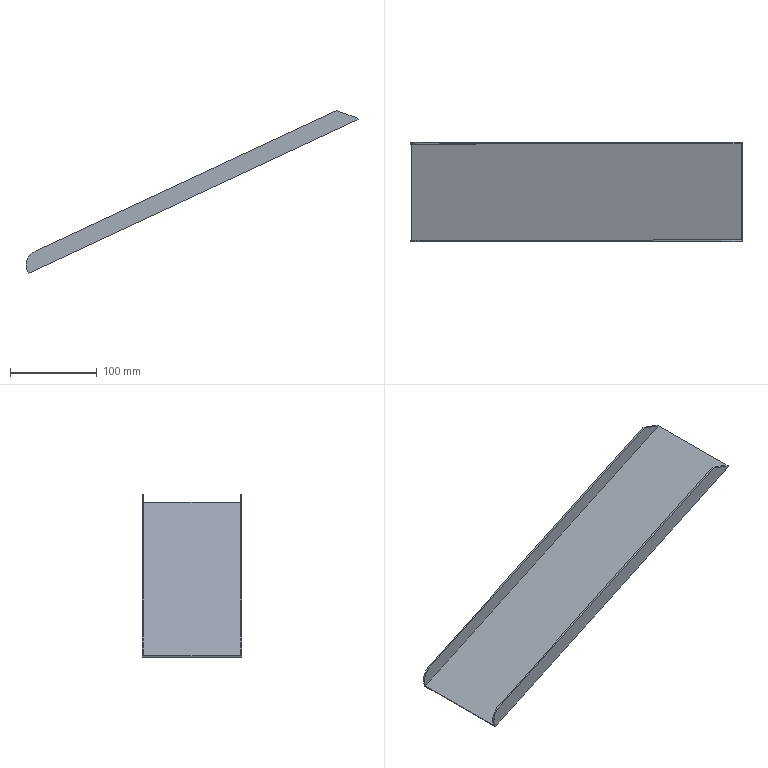Part | NX | features solid 2 | 1 solid | 14 faces | box 383.181 x 115 x 188.019 mm | volume 125914 mm3 | plane 12 | cylinder 2 | commonest cylinder face diameters 36 x2
STEP:
#1=CARTESIAN_POINT('',(-205.649,-420.,-437.5));
#2=VERTEX_POINT('',#1);
#3=CARTESIAN_POINT('',(-204.804,-420.,-439.312));
#4=VERTEX_POINT('',#3);
#5=CARTESIAN_POINT('',(-172.814,-420.,-507.916));
#6=DIRECTION('',(-0.4226,0.,0.9063));
#7=VECTOR('',#6,1000.);
#8=LINE('',#5,#7);
#9=EDGE_CURVE('',#2,#4,#8,.F.);
#10=ORIENTED_EDGE('',*,*,#9,.T.);
#11=CARTESIAN_POINT('',(175.845,-420.,-261.813));
#12=VERTEX_POINT('',#11);
#13=CARTESIAN_POINT('',(-26.99,-420.,-356.396));
#14=DIRECTION('',(0.9063,0.,0.4226));
#15=VECTOR('',#14,1000.);
#16=LINE('',#13,#15);
#17=EDGE_CURVE('',#4,#12,#16,.T.);
#18=ORIENTED_EDGE('',*,*,#17,.T.);
#19=CARTESIAN_POINT('',(175.,-420.,-260.));
#20=VERTEX_POINT('',#19);
#21=CARTESIAN_POINT('',(149.643,-420.,-205.622));
#22=DIRECTION('',(-0.4226,0.,0.9063));
#23=VECTOR('',#22,1000.);
#24=LINE('',#21,#23);
#25=EDGE_CURVE('',#20,#12,#24,.F.);
#26=ORIENTED_EDGE('',*,*,#25,.F.);
#27=CARTESIAN_POINT('',(151.079,-420.,-251.294));
#28=VERTEX_POINT('',#27);
#29=CARTESIAN_POINT('',(-102.746,-420.,-158.909));
#30=DIRECTION('',(0.9397,0.,-0.342));
#31=VECTOR('',#30,1000.);
#32=LINE('',#29,#31);
#33=EDGE_CURVE('',#20,#28,#32,.F.);
#34=ORIENTED_EDGE('',*,*,#33,.T.);
#35=CARTESIAN_POINT('',(-196.943,-420.,-413.579));
#36=VERTEX_POINT('',#35);
#37=CARTESIAN_POINT('',(-213.256,-420.,-421.186));
#38=DIRECTION('',(0.9063,0.,0.4226));
#39=VECTOR('',#38,1000.);
#40=LINE('',#37,#39);
#41=EDGE_CURVE('',#36,#28,#40,.T.);
#42=ORIENTED_EDGE('',*,*,#41,.F.);
#43=CARTESIAN_POINT('',(-189.336,-420.,-429.893));
#44=DIRECTION('',(0.,-1.,0.));
#45=DIRECTION('',(0.,0.,-1.));
#46=AXIS2_PLACEMENT_3D('',#43,#44,#45);
#47=CIRCLE('',#46,18.);
#48=EDGE_CURVE('',#36,#2,#47,.T.);
#49=ORIENTED_EDGE('',*,*,#48,.T.);
#50=EDGE_LOOP('',(#10,#18,#26,#34,#42,#49));
#51=FACE_BOUND('',#50,.T.);
#52=CARTESIAN_POINT('',(5.,-420.,-425.));
#53=DIRECTION('',(0.,1.,0.));
#54=DIRECTION('',(0.,0.,1.));
#55=AXIS2_PLACEMENT_3D('',#52,#53,#54);
#56=PLANE('',#55);
#57=ADVANCED_FACE('',(#51),#56,.F.);
#58=CARTESIAN_POINT('',(175.,-418.,-260.));
#59=VERTEX_POINT('',#58);
#60=CARTESIAN_POINT('',(175.,-307.,-260.));
#61=VERTEX_POINT('',#60);
#62=CARTESIAN_POINT('',(175.,-1000.,-260.));
#63=DIRECTION('',(0.,-1.,0.));
#64=VECTOR('',#63,1000.);
#65=LINE('',#62,#64);
#66=EDGE_CURVE('',#59,#61,#65,.F.);
#67=ORIENTED_EDGE('',*,*,#66,.F.);
#68=CARTESIAN_POINT('',(175.,-1000.,-260.));
#69=DIRECTION('',(0.,-1.,0.));
#70=VECTOR('',#69,1000.);
#71=LINE('',#68,#70);
#72=EDGE_CURVE('',#20,#59,#71,.F.);
#73=ORIENTED_EDGE('',*,*,#72,.F.);
#74=ORIENTED_EDGE('',*,*,#25,.T.);
#75=CARTESIAN_POINT('',(175.845,-305.,-261.813));
#76=VERTEX_POINT('',#75);
#77=CARTESIAN_POINT('',(175.845,-1000.,-261.813));
#78=DIRECTION('',(0.,-1.,0.));
#79=VECTOR('',#78,1000.);
#80=LINE('',#77,#79);
#81=EDGE_CURVE('',#12,#76,#80,.F.);
#82=ORIENTED_EDGE('',*,*,#81,.T.);
#83=CARTESIAN_POINT('',(175.,-305.,-260.));
#84=VERTEX_POINT('',#83);
#85=CARTESIAN_POINT('',(46.966,-305.,14.569));
#86=DIRECTION('',(-0.4226,0.,0.9063));
#87=VECTOR('',#86,1000.);
#88=LINE('',#85,#87);
#89=EDGE_CURVE('',#84,#76,#88,.F.);
#90=ORIENTED_EDGE('',*,*,#89,.F.);
#91=CARTESIAN_POINT('',(175.,-307.,-260.));
#92=DIRECTION('',(0.,-1.,0.));
#93=VECTOR('',#92,1000.);
#94=LINE('',#91,#93);
#95=EDGE_CURVE('',#84,#61,#94,.T.);
#96=ORIENTED_EDGE('',*,*,#95,.T.);
#97=EDGE_LOOP('',(#67,#73,#74,#82,#90,#96));
#98=FACE_BOUND('',#97,.T.);
#99=CARTESIAN_POINT('',(149.643,-1000.,-205.622));
#100=DIRECTION('',(0.9063,0.,0.4226));
#101=DIRECTION('',(-0.4226,0.,0.9063));
#102=AXIS2_PLACEMENT_3D('',#99,#100,#101);
#103=PLANE('',#102);
#104=ADVANCED_FACE('',(#98),#103,.T.);
#105=ORIENTED_EDGE('',*,*,#89,.T.);
#106=CARTESIAN_POINT('',(-204.804,-305.,-439.312));
#107=VERTEX_POINT('',#106);
#108=CARTESIAN_POINT('',(-9.948,-305.,-348.449));
#109=DIRECTION('',(0.9063,0.,0.4226));
#110=VECTOR('',#109,1000.);
#111=LINE('',#108,#110);
#112=EDGE_CURVE('',#107,#76,#111,.T.);
#113=ORIENTED_EDGE('',*,*,#112,.F.);
#114=CARTESIAN_POINT('',(-205.649,-305.,-437.5));
#115=VERTEX_POINT('',#114);
#116=CARTESIAN_POINT('',(-231.006,-305.,-383.121));
#117=DIRECTION('',(-0.4226,0.,0.9063));
#118=VECTOR('',#117,1000.);
#119=LINE('',#116,#118);
#120=EDGE_CURVE('',#115,#107,#119,.F.);
#121=ORIENTED_EDGE('',*,*,#120,.F.);
#122=CARTESIAN_POINT('',(-196.943,-305.,-413.579));
#123=VERTEX_POINT('',#122);
#124=CARTESIAN_POINT('',(-189.336,-305.,-429.893));
#125=DIRECTION('',(0.,1.,0.));
#126=DIRECTION('',(0.,0.,1.));
#127=AXIS2_PLACEMENT_3D('',#124,#125,#126);
#128=CIRCLE('',#127,18.);
#129=EDGE_CURVE('',#115,#123,#128,.T.);
#130=ORIENTED_EDGE('',*,*,#129,.T.);
#131=CARTESIAN_POINT('',(151.079,-305.,-251.294));
#132=VERTEX_POINT('',#131);
#133=CARTESIAN_POINT('',(-213.256,-305.,-421.186));
#134=DIRECTION('',(-0.9063,0.,-0.4226));
#135=VECTOR('',#134,1000.);
#136=LINE('',#133,#135);
#137=EDGE_CURVE('',#123,#132,#136,.F.);
#138=ORIENTED_EDGE('',*,*,#137,.T.);
#139=CARTESIAN_POINT('',(-102.746,-305.,-158.909));
#140=DIRECTION('',(0.9397,0.,-0.342));
#141=VECTOR('',#140,1000.);
#142=LINE('',#139,#141);
#143=EDGE_CURVE('',#132,#84,#142,.T.);
#144=ORIENTED_EDGE('',*,*,#143,.T.);
#145=EDGE_LOOP('',(#105,#113,#121,#130,#138,#144));
#146=FACE_BOUND('',#145,.T.);
#147=CARTESIAN_POINT('',(5.,-305.,-5.));
#148=DIRECTION('',(0.,-1.,0.));
#149=DIRECTION('',(0.,0.,-1.));
#150=AXIS2_PLACEMENT_3D('',#147,#148,#149);
#151=PLANE('',#150);
#152=ADVANCED_FACE('',(#146),#151,.F.);
#153=ORIENTED_EDGE('',*,*,#120,.T.);
#154=CARTESIAN_POINT('',(-204.804,-420.,-439.312));
#155=DIRECTION('',(0.,-1.,0.));
#156=VECTOR('',#155,1000.);
#157=LINE('',#154,#156);
#158=EDGE_CURVE('',#4,#107,#157,.F.);
#159=ORIENTED_EDGE('',*,*,#158,.F.);
#160=ORIENTED_EDGE('',*,*,#9,.F.);
#161=CARTESIAN_POINT('',(-205.649,-418.,-437.5));
#162=VERTEX_POINT('',#161);
#163=CARTESIAN_POINT('',(-205.649,-420.,-437.5));
#164=DIRECTION('',(0.,-1.,0.));
#165=VECTOR('',#164,1000.);
#166=LINE('',#163,#165);
#167=EDGE_CURVE('',#2,#162,#166,.F.);
#168=ORIENTED_EDGE('',*,*,#167,.T.);
#169=CARTESIAN_POINT('',(-205.649,-307.,-437.5));
#170=VERTEX_POINT('',#169);
#171=CARTESIAN_POINT('',(-205.649,-420.,-437.5));
#172=DIRECTION('',(0.,-1.,0.));
#173=VECTOR('',#172,1000.);
#174=LINE('',#171,#173);
#175=EDGE_CURVE('',#162,#170,#174,.F.);
#176=ORIENTED_EDGE('',*,*,#175,.T.);
#177=CARTESIAN_POINT('',(-205.649,-305.,-437.5));
#178=DIRECTION('',(0.,-1.,0.));
#179=VECTOR('',#178,1000.);
#180=LINE('',#177,#179);
#181=EDGE_CURVE('',#170,#115,#180,.F.);
#182=ORIENTED_EDGE('',*,*,#181,.T.);
#183=EDGE_LOOP('',(#153,#159,#160,#168,#176,#182));
#184=FACE_BOUND('',#183,.T.);
#185=CARTESIAN_POINT('',(-231.006,-1000.,-383.121));
#186=DIRECTION('',(-0.9063,0.,-0.4226));
#187=DIRECTION('',(0.4226,0.,-0.9063));
#188=AXIS2_PLACEMENT_3D('',#185,#186,#187);
#189=PLANE('',#188);
#190=ADVANCED_FACE('',(#184),#189,.T.);
#191=ORIENTED_EDGE('',*,*,#112,.T.);
#192=ORIENTED_EDGE('',*,*,#81,.F.);
#193=ORIENTED_EDGE('',*,*,#17,.F.);
#194=ORIENTED_EDGE('',*,*,#158,.T.);
#195=EDGE_LOOP('',(#191,#192,#193,#194));
#196=FACE_BOUND('',#195,.T.);
#197=CARTESIAN_POINT('',(-9.948,-420.,-348.449));
#198=DIRECTION('',(-0.4226,0.,0.9063));
#199=DIRECTION('',(0.9063,0.,0.4226));
#200=AXIS2_PLACEMENT_3D('',#197,#198,#199);
#201=PLANE('',#200);
#202=ADVANCED_FACE('',(#196),#201,.F.);
#203=CARTESIAN_POINT('',(-10.793,-418.,-346.637));
#204=DIRECTION('',(0.9063,0.,0.4226));
#205=VECTOR('',#204,1000.);
#206=LINE('',#203,#205);
#207=EDGE_CURVE('',#59,#162,#206,.F.);
#208=ORIENTED_EDGE('',*,*,#207,.F.);
#209=ORIENTED_EDGE('',*,*,#66,.T.);
#210=CARTESIAN_POINT('',(-10.793,-307.,-346.637));
#211=DIRECTION('',(-0.9063,0.,-0.4226));
#212=VECTOR('',#211,1000.);
#213=LINE('',#210,#212);
#214=EDGE_CURVE('',#170,#61,#213,.F.);
#215=ORIENTED_EDGE('',*,*,#214,.F.);
#216=ORIENTED_EDGE('',*,*,#175,.F.);
#217=EDGE_LOOP('',(#208,#209,#215,#216));
#218=FACE_BOUND('',#217,.T.);
#219=CARTESIAN_POINT('',(-10.793,-420.,-346.637));
#220=DIRECTION('',(-0.4226,0.,0.9063));
#221=DIRECTION('',(0.9063,0.,0.4226));
#222=AXIS2_PLACEMENT_3D('',#219,#220,#221);
#223=PLANE('',#222);
#224=ADVANCED_FACE('',(#218),#223,.T.);
#225=CARTESIAN_POINT('',(-196.943,-307.,-413.579));
#226=VERTEX_POINT('',#225);
#227=CARTESIAN_POINT('',(-189.336,-307.,-429.893));
#228=DIRECTION('',(0.,1.,0.));
#229=DIRECTION('',(0.,0.,1.));
#230=AXIS2_PLACEMENT_3D('',#227,#228,#229);
#231=CIRCLE('',#230,18.);
#232=EDGE_CURVE('',#226,#170,#231,.F.);
#233=ORIENTED_EDGE('',*,*,#232,.T.);
#234=ORIENTED_EDGE('',*,*,#214,.T.);
#235=CARTESIAN_POINT('',(151.079,-307.,-251.294));
#236=VERTEX_POINT('',#235);
#237=CARTESIAN_POINT('',(-102.746,-307.,-158.909));
#238=DIRECTION('',(0.9397,0.,-0.342));
#239=VECTOR('',#238,1000.);
#240=LINE('',#237,#239);
#241=EDGE_CURVE('',#61,#236,#240,.F.);
#242=ORIENTED_EDGE('',*,*,#241,.T.);
#243=CARTESIAN_POINT('',(-213.256,-307.,-421.186));
#244=DIRECTION('',(-0.9063,0.,-0.4226));
#245=VECTOR('',#244,1000.);
#246=LINE('',#243,#245);
#247=EDGE_CURVE('',#226,#236,#246,.F.);
#248=ORIENTED_EDGE('',*,*,#247,.F.);
#249=EDGE_LOOP('',(#233,#234,#242,#248));
#250=FACE_BOUND('',#249,.T.);
#251=CARTESIAN_POINT('',(-204.804,-307.,-439.312));
#252=DIRECTION('',(0.,1.,0.));
#253=DIRECTION('',(0.9063,0.,0.4226));
#254=AXIS2_PLACEMENT_3D('',#251,#252,#253);
#255=PLANE('',#254);
#256=ADVANCED_FACE('',(#250),#255,.F.);
#257=ORIENTED_EDGE('',*,*,#247,.T.);
#258=CARTESIAN_POINT('',(151.079,-305.,-251.294));
#259=DIRECTION('',(0.,1.,0.));
#260=VECTOR('',#259,1000.);
#261=LINE('',#258,#260);
#262=EDGE_CURVE('',#236,#132,#261,.T.);
#263=ORIENTED_EDGE('',*,*,#262,.T.);
#264=ORIENTED_EDGE('',*,*,#137,.F.);
#265=CARTESIAN_POINT('',(-196.943,-307.,-413.579));
#266=DIRECTION('',(0.,1.,0.));
#267=VECTOR('',#266,1000.);
#268=LINE('',#265,#267);
#269=EDGE_CURVE('',#123,#226,#268,.F.);
#270=ORIENTED_EDGE('',*,*,#269,.T.);
#271=EDGE_LOOP('',(#257,#263,#264,#270));
#272=FACE_BOUND('',#271,.T.);
#273=CARTESIAN_POINT('',(-213.256,-305.,-421.186));
#274=DIRECTION('',(0.4226,0.,-0.9063));
#275=DIRECTION('',(-0.9063,0.,-0.4226));
#276=AXIS2_PLACEMENT_3D('',#273,#274,#275);
#277=PLANE('',#276);
#278=ADVANCED_FACE('',(#272),#277,.F.);
#279=ORIENTED_EDGE('',*,*,#129,.F.);
#280=ORIENTED_EDGE('',*,*,#181,.F.);
#281=ORIENTED_EDGE('',*,*,#232,.F.);
#282=ORIENTED_EDGE('',*,*,#269,.F.);
#283=EDGE_LOOP('',(#279,#280,#281,#282));
#284=FACE_BOUND('',#283,.T.);
#285=CARTESIAN_POINT('',(-189.336,-305.,-429.893));
#286=DIRECTION('',(0.,-1.,0.));
#287=DIRECTION('',(0.,0.,-1.));
#288=AXIS2_PLACEMENT_3D('',#285,#286,#287);
#289=CYLINDRICAL_SURFACE('',#288,18.);
#290=ADVANCED_FACE('',(#284),#289,.T.);
#291=ORIENTED_EDGE('',*,*,#143,.F.);
#292=ORIENTED_EDGE('',*,*,#262,.F.);
#293=ORIENTED_EDGE('',*,*,#241,.F.);
#294=ORIENTED_EDGE('',*,*,#95,.F.);
#295=EDGE_LOOP('',(#291,#292,#293,#294));
#296=FACE_BOUND('',#295,.T.);
#297=CARTESIAN_POINT('',(175.,-305.,-260.));
#298=DIRECTION('',(0.342,0.,0.9397));
#299=DIRECTION('',(0.9397,0.,-0.342));
#300=AXIS2_PLACEMENT_3D('',#297,#298,#299);
#301=PLANE('',#300);
#302=ADVANCED_FACE('',(#296),#301,.T.);
#303=CARTESIAN_POINT('',(151.079,-418.,-251.294));
#304=VERTEX_POINT('',#303);
#305=CARTESIAN_POINT('',(-102.746,-418.,-158.909));
#306=DIRECTION('',(0.9397,0.,-0.342));
#307=VECTOR('',#306,1000.);
#308=LINE('',#305,#307);
#309=EDGE_CURVE('',#304,#59,#308,.T.);
#310=ORIENTED_EDGE('',*,*,#309,.T.);
#311=ORIENTED_EDGE('',*,*,#207,.T.);
#312=CARTESIAN_POINT('',(-196.943,-418.,-413.579));
#313=VERTEX_POINT('',#312);
#314=CARTESIAN_POINT('',(-189.336,-418.,-429.893));
#315=DIRECTION('',(0.,-1.,0.));
#316=DIRECTION('',(0.,0.,-1.));
#317=AXIS2_PLACEMENT_3D('',#314,#315,#316);
#318=CIRCLE('',#317,18.);
#319=EDGE_CURVE('',#162,#313,#318,.F.);
#320=ORIENTED_EDGE('',*,*,#319,.T.);
#321=CARTESIAN_POINT('',(-213.256,-418.,-421.186));
#322=DIRECTION('',(0.9063,0.,0.4226));
#323=VECTOR('',#322,1000.);
#324=LINE('',#321,#323);
#325=EDGE_CURVE('',#313,#304,#324,.T.);
#326=ORIENTED_EDGE('',*,*,#325,.T.);
#327=EDGE_LOOP('',(#310,#311,#320,#326));
#328=FACE_BOUND('',#327,.T.);
#329=CARTESIAN_POINT('',(-204.804,-418.,-439.312));
#330=DIRECTION('',(0.,-1.,0.));
#331=DIRECTION('',(0.9063,0.,0.4226));
#332=AXIS2_PLACEMENT_3D('',#329,#330,#331);
#333=PLANE('',#332);
#334=ADVANCED_FACE('',(#328),#333,.F.);
#335=ORIENTED_EDGE('',*,*,#41,.T.);
#336=CARTESIAN_POINT('',(151.079,-420.,-251.294));
#337=DIRECTION('',(0.,1.,0.));
#338=VECTOR('',#337,1000.);
#339=LINE('',#336,#338);
#340=EDGE_CURVE('',#28,#304,#339,.T.);
#341=ORIENTED_EDGE('',*,*,#340,.T.);
#342=ORIENTED_EDGE('',*,*,#325,.F.);
#343=CARTESIAN_POINT('',(-196.943,-420.,-413.579));
#344=DIRECTION('',(0.,-1.,0.));
#345=VECTOR('',#344,1000.);
#346=LINE('',#343,#345);
#347=EDGE_CURVE('',#313,#36,#346,.T.);
#348=ORIENTED_EDGE('',*,*,#347,.T.);
#349=EDGE_LOOP('',(#335,#341,#342,#348));
#350=FACE_BOUND('',#349,.T.);
#351=CARTESIAN_POINT('',(-213.256,-420.,-421.186));
#352=DIRECTION('',(-0.4226,0.,0.9063));
#353=DIRECTION('',(0.9063,0.,0.4226));
#354=AXIS2_PLACEMENT_3D('',#351,#352,#353);
#355=PLANE('',#354);
#356=ADVANCED_FACE('',(#350),#355,.T.);
#357=ORIENTED_EDGE('',*,*,#48,.F.);
#358=ORIENTED_EDGE('',*,*,#347,.F.);
#359=ORIENTED_EDGE('',*,*,#319,.F.);
#360=ORIENTED_EDGE('',*,*,#167,.F.);
#361=EDGE_LOOP('',(#357,#358,#359,#360));
#362=FACE_BOUND('',#361,.T.);
#363=CARTESIAN_POINT('',(-189.336,-420.,-429.893));
#364=DIRECTION('',(0.,-1.,0.));
#365=DIRECTION('',(0.,0.,-1.));
#366=AXIS2_PLACEMENT_3D('',#363,#364,#365);
#367=CYLINDRICAL_SURFACE('',#366,18.);
#368=ADVANCED_FACE('',(#362),#367,.T.);
#369=ORIENTED_EDGE('',*,*,#33,.F.);
#370=ORIENTED_EDGE('',*,*,#72,.T.);
#371=ORIENTED_EDGE('',*,*,#309,.F.);
#372=ORIENTED_EDGE('',*,*,#340,.F.);
#373=EDGE_LOOP('',(#369,#370,#371,#372));
#374=FACE_BOUND('',#373,.T.);
#375=CARTESIAN_POINT('',(151.079,-420.,-251.294));
#376=DIRECTION('',(-0.342,0.,-0.9397));
#377=DIRECTION('',(-0.9397,0.,0.342));
#378=AXIS2_PLACEMENT_3D('',#375,#376,#377);
#379=PLANE('',#378);
#380=ADVANCED_FACE('',(#374),#379,.F.);
#381=CLOSED_SHELL('',(#57,#104,#152,#190,#202,#224,#256,#278,#290,#302,#334,#356,#368,#380));
#382=MANIFOLD_SOLID_BREP('',#381);
#383=(LENGTH_UNIT()NAMED_UNIT(*)SI_UNIT(.MILLI.,.METRE.));
#384=UNCERTAINTY_MEASURE_WITH_UNIT(LENGTH_MEASURE(0.00001),#383,'','');
#385=(NAMED_UNIT(*)PLANE_ANGLE_UNIT()SI_UNIT($,.RADIAN.));
#386=(NAMED_UNIT(*)SI_UNIT($,.STERADIAN.)SOLID_ANGLE_UNIT());
#387=(GEOMETRIC_REPRESENTATION_CONTEXT(3)GLOBAL_UNCERTAINTY_ASSIGNED_CONTEXT((#384))GLOBAL_UNIT_ASSIGNED_CONTEXT((#383,#385,#386))REPRESENTATION_CONTEXT('',''));
#388=ADVANCED_BREP_SHAPE_REPRESENTATION('',(#382),#387);